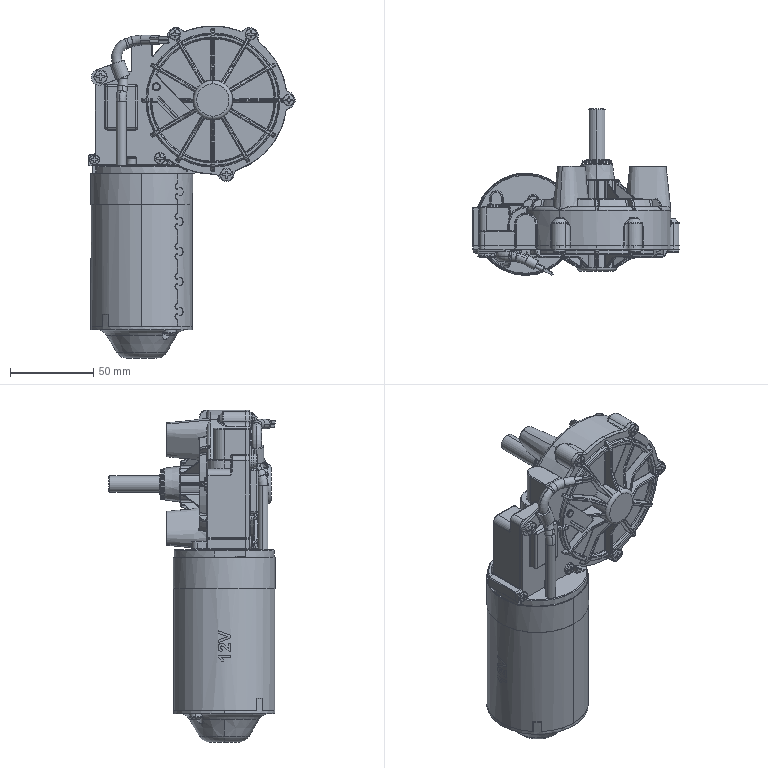Part | STEP file | Gear motor - 12V (6 holes)_Default | 20 solids | 2923 faces | box 124.05 x 100.1 x 199.5 mm | volume 340663 mm3 | cylinder 960 | spline 666 | torus 583 | plane 511 | sphere 102 | cone 101 | commonest cylinder face diameters 0.4 x242 1 x167 2 x69 0.2 x63 0.1 x61 10 x27